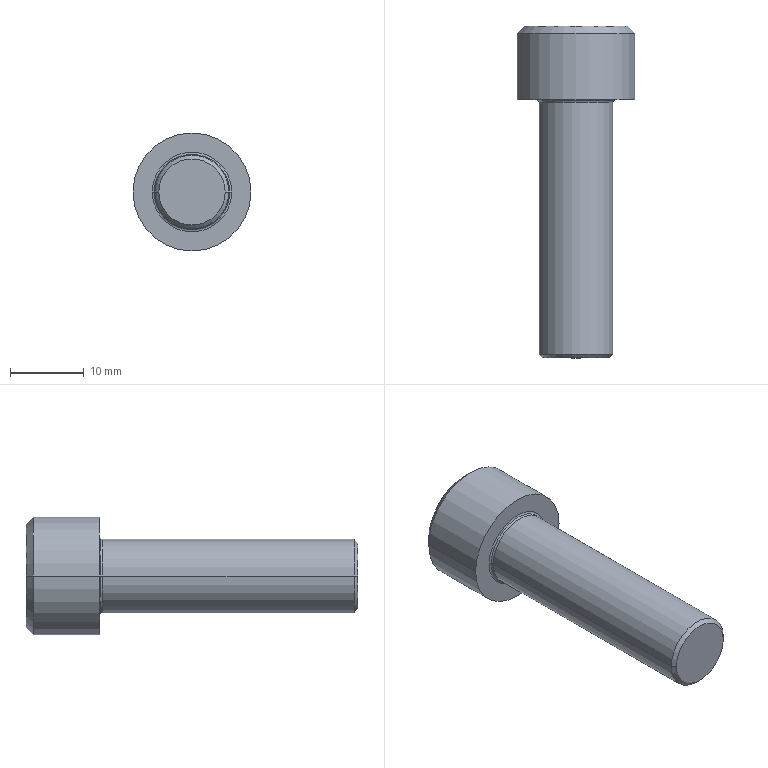Part | Creo | 1 solid | 23 faces | box 16 x 45 x 16 mm | volume 4398 mm3 | plane 9 | cone 6 | cylinder 4 | torus 4 | commonest cylinder face diameters 10 x2 16 x2
STEP:
#1=CARTESIAN_POINT('',(-187.881,357.995,-225.));
#2=VERTEX_POINT('',#1);
#3=CARTESIAN_POINT('',(-190.191,357.995,-229.));
#4=VERTEX_POINT('',#3);
#5=CARTESIAN_POINT('',(-187.881,357.995,-225.));
#6=CARTESIAN_POINT('',(-187.989,357.933,-225.187));
#7=CARTESIAN_POINT('',(-188.205,357.821,-225.561));
#8=CARTESIAN_POINT('',(-188.534,357.7,-226.131));
#9=CARTESIAN_POINT('',(-188.867,357.635,-226.708));
#10=CARTESIAN_POINT('',(-189.204,357.635,-227.29));
#11=CARTESIAN_POINT('',(-189.537,357.7,-227.868));
#12=CARTESIAN_POINT('',(-189.865,357.821,-228.437));
#13=CARTESIAN_POINT('',(-190.082,357.933,-228.813));
#14=CARTESIAN_POINT('',(-190.191,357.995,-229.));
#15=B_SPLINE_CURVE_WITH_KNOTS('',3,(#5,#6,#7,#8,#9,#10,#11,#12,#13,#14),.UNSPECIFIED.,.F.,.F.,(4,1,1,1,1,1,1,4),(0.,0.1429,0.2857,0.4286,0.5714,0.7143,0.8571,1.),.UNSPECIFIED.);
#16=EDGE_CURVE('',#2,#4,#15,.T.);
#17=ORIENTED_EDGE('',*,*,#16,.F.);
#18=CARTESIAN_POINT('',(-192.5,355.329,-225.));
#19=VERTEX_POINT('',#18);
#20=CARTESIAN_POINT('',(-192.5,355.329,-225.));
#21=DIRECTION('',(0.866,0.5,0.));
#22=VECTOR('',#21,5.333);
#23=LINE('',#20,#22);
#24=EDGE_CURVE('',#19,#2,#23,.T.);
#25=ORIENTED_EDGE('',*,*,#24,.F.);
#26=CARTESIAN_POINT('',(-197.119,357.995,-225.));
#27=VERTEX_POINT('',#26);
#28=CARTESIAN_POINT('',(-192.5,355.329,-225.));
#29=DIRECTION('',(-0.866,0.5,0.));
#30=VECTOR('',#29,5.333);
#31=LINE('',#28,#30);
#32=EDGE_CURVE('',#19,#27,#31,.T.);
#33=ORIENTED_EDGE('',*,*,#32,.T.);
#34=CARTESIAN_POINT('',(-194.809,357.995,-229.));
#35=VERTEX_POINT('',#34);
#36=CARTESIAN_POINT('',(-194.809,357.995,-229.));
#37=CARTESIAN_POINT('',(-194.917,357.933,-228.813));
#38=CARTESIAN_POINT('',(-195.133,357.821,-228.439));
#39=CARTESIAN_POINT('',(-195.462,357.7,-227.869));
#40=CARTESIAN_POINT('',(-195.795,357.635,-227.292));
#41=CARTESIAN_POINT('',(-196.132,357.635,-226.71));
#42=CARTESIAN_POINT('',(-196.465,357.7,-226.132));
#43=CARTESIAN_POINT('',(-196.794,357.821,-225.563));
#44=CARTESIAN_POINT('',(-197.011,357.933,-225.187));
#45=CARTESIAN_POINT('',(-197.119,357.995,-225.));
#46=B_SPLINE_CURVE_WITH_KNOTS('',3,(#36,#37,#38,#39,#40,#41,#42,#43,#44,#45),.UNSPECIFIED.,.F.,.F.,(4,1,1,1,1,1,1,4),(0.,0.1429,0.2857,0.4286,0.5714,0.7143,0.8571,1.),.UNSPECIFIED.);
#47=EDGE_CURVE('',#35,#27,#46,.T.);
#48=ORIENTED_EDGE('',*,*,#47,.F.);
#49=CARTESIAN_POINT('',(-190.191,357.995,-229.));
#50=CARTESIAN_POINT('',(-190.404,357.934,-229.));
#51=CARTESIAN_POINT('',(-190.835,357.822,-229.));
#52=CARTESIAN_POINT('',(-191.496,357.7,-229.));
#53=CARTESIAN_POINT('',(-192.165,357.635,-229.));
#54=CARTESIAN_POINT('',(-192.833,357.635,-229.));
#55=CARTESIAN_POINT('',(-193.5,357.699,-229.));
#56=CARTESIAN_POINT('',(-194.162,357.821,-229.));
#57=CARTESIAN_POINT('',(-194.594,357.933,-229.));
#58=CARTESIAN_POINT('',(-194.809,357.995,-229.));
#59=B_SPLINE_CURVE_WITH_KNOTS('',3,(#49,#50,#51,#52,#53,#54,#55,#56,#57,#58),.UNSPECIFIED.,.F.,.F.,(4,1,1,1,1,1,1,4),(0.,0.1429,0.2857,0.4286,0.5714,0.7143,0.8571,1.),.UNSPECIFIED.);
#60=EDGE_CURVE('',#4,#35,#59,.T.);
#61=ORIENTED_EDGE('',*,*,#60,.F.);
#62=EDGE_LOOP('',(#17,#25,#33,#48,#61));
#63=FACE_OUTER_BOUND('',#62,.F.);
#64=CARTESIAN_POINT('',(-192.5,356.689,-225.));
#65=DIRECTION('',(0.,1.,0.));
#66=DIRECTION('',(1.,0.,0.));
#67=AXIS2_PLACEMENT_3D('',#64,#65,#66);
#68=CONICAL_SURFACE('',#67,2.356,60.);
#69=ADVANCED_FACE('',(#63),#68,.F.);
#70=CARTESIAN_POINT('',(-190.191,362.995,-229.));
#71=VERTEX_POINT('',#70);
#72=CARTESIAN_POINT('',(-187.881,362.995,-225.));
#73=VERTEX_POINT('',#72);
#74=CARTESIAN_POINT('',(-190.191,362.995,-229.));
#75=DIRECTION('',(0.5,0.,0.866));
#76=VECTOR('',#75,4.619);
#77=LINE('',#74,#76);
#78=EDGE_CURVE('',#71,#73,#77,.T.);
#79=ORIENTED_EDGE('',*,*,#78,.T.);
#80=CARTESIAN_POINT('',(-187.881,362.995,-225.));
#81=DIRECTION('',(0.,-1.,0.));
#82=VECTOR('',#81,5.);
#83=LINE('',#80,#82);
#84=EDGE_CURVE('',#73,#2,#83,.T.);
#85=ORIENTED_EDGE('',*,*,#84,.T.);
#86=ORIENTED_EDGE('',*,*,#16,.T.);
#87=CARTESIAN_POINT('',(-190.191,362.995,-229.));
#88=DIRECTION('',(0.,-1.,0.));
#89=VECTOR('',#88,5.);
#90=LINE('',#87,#89);
#91=EDGE_CURVE('',#71,#4,#90,.T.);
#92=ORIENTED_EDGE('',*,*,#91,.F.);
#93=EDGE_LOOP('',(#79,#85,#86,#92));
#94=FACE_OUTER_BOUND('',#93,.F.);
#95=CARTESIAN_POINT('',(-190.191,357.995,-229.));
#96=DIRECTION('',(-0.866,0.,0.5));
#97=DIRECTION('',(0.5,0.,0.866));
#98=AXIS2_PLACEMENT_3D('',#95,#96,#97);
#99=PLANE('',#98);
#100=ADVANCED_FACE('',(#94),#99,.T.);
#101=CARTESIAN_POINT('',(-185.5,362.995,-225.));
#102=VERTEX_POINT('',#101);
#103=CARTESIAN_POINT('',(-199.5,362.995,-225.));
#104=VERTEX_POINT('',#103);
#105=CARTESIAN_POINT('',(-192.5,362.995,-225.));
#106=DIRECTION('',(0.,1.,0.));
#107=DIRECTION('',(1.,0.,0.));
#108=AXIS2_PLACEMENT_3D('',#105,#106,#107);
#109=CIRCLE('',#108,7.);
#110=EDGE_CURVE('',#102,#104,#109,.T.);
#111=ORIENTED_EDGE('',*,*,#110,.F.);
#112=CARTESIAN_POINT('',(-192.5,362.995,-225.));
#113=DIRECTION('',(0.,1.,0.));
#114=DIRECTION('',(-1.,0.,0.));
#115=AXIS2_PLACEMENT_3D('',#112,#113,#114);
#116=CIRCLE('',#115,7.);
#117=EDGE_CURVE('',#104,#102,#116,.T.);
#118=ORIENTED_EDGE('',*,*,#117,.F.);
#119=EDGE_LOOP('',(#111,#118));
#120=FACE_OUTER_BOUND('',#119,.F.);
#121=CARTESIAN_POINT('',(-190.191,362.995,-221.));
#122=VERTEX_POINT('',#121);
#123=CARTESIAN_POINT('',(-187.881,362.995,-225.));
#124=DIRECTION('',(-0.5,0.,0.866));
#125=VECTOR('',#124,4.619);
#126=LINE('',#123,#125);
#127=EDGE_CURVE('',#73,#122,#126,.T.);
#128=ORIENTED_EDGE('',*,*,#127,.F.);
#129=ORIENTED_EDGE('',*,*,#78,.F.);
#130=CARTESIAN_POINT('',(-194.809,362.995,-229.));
#131=VERTEX_POINT('',#130);
#132=CARTESIAN_POINT('',(-190.191,362.995,-229.));
#133=DIRECTION('',(-1.,0.,0.));
#134=VECTOR('',#133,4.619);
#135=LINE('',#132,#134);
#136=EDGE_CURVE('',#71,#131,#135,.T.);
#137=ORIENTED_EDGE('',*,*,#136,.T.);
#138=CARTESIAN_POINT('',(-197.119,362.995,-225.));
#139=VERTEX_POINT('',#138);
#140=CARTESIAN_POINT('',(-197.119,362.995,-225.));
#141=DIRECTION('',(0.5,0.,-0.866));
#142=VECTOR('',#141,4.619);
#143=LINE('',#140,#142);
#144=EDGE_CURVE('',#139,#131,#143,.T.);
#145=ORIENTED_EDGE('',*,*,#144,.F.);
#146=CARTESIAN_POINT('',(-194.809,362.995,-221.));
#147=VERTEX_POINT('',#146);
#148=CARTESIAN_POINT('',(-194.809,362.995,-221.));
#149=DIRECTION('',(-0.5,0.,-0.866));
#150=VECTOR('',#149,4.619);
#151=LINE('',#148,#150);
#152=EDGE_CURVE('',#147,#139,#151,.T.);
#153=ORIENTED_EDGE('',*,*,#152,.F.);
#154=CARTESIAN_POINT('',(-194.809,362.995,-221.));
#155=DIRECTION('',(1.,0.,0.));
#156=VECTOR('',#155,4.619);
#157=LINE('',#154,#156);
#158=EDGE_CURVE('',#147,#122,#157,.T.);
#159=ORIENTED_EDGE('',*,*,#158,.T.);
#160=EDGE_LOOP('',(#128,#129,#137,#145,#153,#159));
#161=FACE_BOUND('',#160,.F.);
#162=CARTESIAN_POINT('',(-192.5,362.995,-225.));
#163=DIRECTION('',(0.,1.,0.));
#164=DIRECTION('',(1.,0.,0.));
#165=AXIS2_PLACEMENT_3D('',#162,#163,#164);
#166=PLANE('',#165);
#167=ADVANCED_FACE('',(#120,#161),#166,.T.);
#168=CARTESIAN_POINT('',(-184.5,361.995,-225.));
#169=VERTEX_POINT('',#168);
#170=CARTESIAN_POINT('',(-200.5,361.995,-225.));
#171=VERTEX_POINT('',#170);
#172=CARTESIAN_POINT('',(-192.5,361.995,-225.));
#173=DIRECTION('',(0.,1.,0.));
#174=DIRECTION('',(1.,0.,0.));
#175=AXIS2_PLACEMENT_3D('',#172,#173,#174);
#176=CIRCLE('',#175,8.);
#177=EDGE_CURVE('',#169,#171,#176,.T.);
#178=ORIENTED_EDGE('',*,*,#177,.F.);
#179=CARTESIAN_POINT('',(-185.5,362.995,-225.));
#180=DIRECTION('',(0.7071,-0.7071,0.));
#181=VECTOR('',#180,1.414);
#182=LINE('',#179,#181);
#183=EDGE_CURVE('',#102,#169,#182,.T.);
#184=ORIENTED_EDGE('',*,*,#183,.F.);
#185=ORIENTED_EDGE('',*,*,#110,.T.);
#186=CARTESIAN_POINT('',(-199.5,362.995,-225.));
#187=DIRECTION('',(-0.7071,-0.7071,0.));
#188=VECTOR('',#187,1.414);
#189=LINE('',#186,#188);
#190=EDGE_CURVE('',#104,#171,#189,.T.);
#191=ORIENTED_EDGE('',*,*,#190,.T.);
#192=EDGE_LOOP('',(#178,#184,#185,#191));
#193=FACE_OUTER_BOUND('',#192,.F.);
#194=CARTESIAN_POINT('',(-192.5,362.495,-225.));
#195=DIRECTION('',(0.,-1.,0.));
#196=DIRECTION('',(-1.,0.,0.));
#197=AXIS2_PLACEMENT_3D('',#194,#195,#196);
#198=CONICAL_SURFACE('',#197,7.5,45.);
#199=ADVANCED_FACE('',(#193),#198,.T.);
#200=ORIENTED_EDGE('',*,*,#177,.T.);
#201=CARTESIAN_POINT('',(-200.5,352.995,-225.));
#202=VERTEX_POINT('',#201);
#203=CARTESIAN_POINT('',(-200.5,352.995,-225.));
#204=DIRECTION('',(0.,1.,0.));
#205=VECTOR('',#204,9.);
#206=LINE('',#203,#205);
#207=EDGE_CURVE('',#202,#171,#206,.T.);
#208=ORIENTED_EDGE('',*,*,#207,.F.);
#209=CARTESIAN_POINT('',(-184.5,352.995,-225.));
#210=VERTEX_POINT('',#209);
#211=CARTESIAN_POINT('',(-192.5,352.995,-225.));
#212=DIRECTION('',(0.,-1.,0.));
#213=DIRECTION('',(-1.,0.,0.));
#214=AXIS2_PLACEMENT_3D('',#211,#212,#213);
#215=CIRCLE('',#214,8.);
#216=EDGE_CURVE('',#202,#210,#215,.T.);
#217=ORIENTED_EDGE('',*,*,#216,.T.);
#218=CARTESIAN_POINT('',(-184.5,352.995,-225.));
#219=DIRECTION('',(0.,1.,0.));
#220=VECTOR('',#219,9.);
#221=LINE('',#218,#220);
#222=EDGE_CURVE('',#210,#169,#221,.T.);
#223=ORIENTED_EDGE('',*,*,#222,.T.);
#224=EDGE_LOOP('',(#200,#208,#217,#223));
#225=FACE_OUTER_BOUND('',#224,.F.);
#226=CARTESIAN_POINT('',(-192.5,352.995,-225.));
#227=DIRECTION('',(0.,1.,0.));
#228=DIRECTION('',(1.,0.,0.));
#229=AXIS2_PLACEMENT_3D('',#226,#227,#228);
#230=CYLINDRICAL_SURFACE('',#229,8.);
#231=ADVANCED_FACE('',(#225),#230,.T.);
#232=CARTESIAN_POINT('',(-192.5,361.995,-225.));
#233=DIRECTION('',(0.,1.,0.));
#234=DIRECTION('',(-1.,0.,0.));
#235=AXIS2_PLACEMENT_3D('',#232,#233,#234);
#236=CIRCLE('',#235,8.);
#237=EDGE_CURVE('',#171,#169,#236,.T.);
#238=ORIENTED_EDGE('',*,*,#237,.T.);
#239=ORIENTED_EDGE('',*,*,#222,.F.);
#240=CARTESIAN_POINT('',(-192.5,352.995,-225.));
#241=DIRECTION('',(0.,-1.,0.));
#242=DIRECTION('',(1.,0.,0.));
#243=AXIS2_PLACEMENT_3D('',#240,#241,#242);
#244=CIRCLE('',#243,8.);
#245=EDGE_CURVE('',#210,#202,#244,.T.);
#246=ORIENTED_EDGE('',*,*,#245,.T.);
#247=ORIENTED_EDGE('',*,*,#207,.T.);
#248=EDGE_LOOP('',(#238,#239,#246,#247));
#249=FACE_OUTER_BOUND('',#248,.F.);
#250=CARTESIAN_POINT('',(-192.5,352.995,-225.));
#251=DIRECTION('',(0.,1.,0.));
#252=DIRECTION('',(1.,0.,0.));
#253=AXIS2_PLACEMENT_3D('',#250,#251,#252);
#254=CYLINDRICAL_SURFACE('',#253,8.);
#255=ADVANCED_FACE('',(#249),#254,.T.);
#256=ORIENTED_EDGE('',*,*,#237,.F.);
#257=ORIENTED_EDGE('',*,*,#190,.F.);
#258=ORIENTED_EDGE('',*,*,#117,.T.);
#259=ORIENTED_EDGE('',*,*,#183,.T.);
#260=EDGE_LOOP('',(#256,#257,#258,#259));
#261=FACE_OUTER_BOUND('',#260,.F.);
#262=CARTESIAN_POINT('',(-192.5,362.495,-225.));
#263=DIRECTION('',(0.,-1.,0.));
#264=DIRECTION('',(-1.,0.,0.));
#265=AXIS2_PLACEMENT_3D('',#262,#263,#264);
#266=CONICAL_SURFACE('',#265,7.5,45.);
#267=ADVANCED_FACE('',(#261),#266,.T.);
#268=ORIENTED_EDGE('',*,*,#245,.F.);
#269=ORIENTED_EDGE('',*,*,#216,.F.);
#270=EDGE_LOOP('',(#268,#269));
#271=FACE_OUTER_BOUND('',#270,.F.);
#272=CARTESIAN_POINT('',(-187.1,352.995,-225.));
#273=VERTEX_POINT('',#272);
#274=CARTESIAN_POINT('',(-197.9,352.995,-225.));
#275=VERTEX_POINT('',#274);
#276=CARTESIAN_POINT('',(-192.5,352.995,-225.));
#277=DIRECTION('',(0.,1.,0.));
#278=DIRECTION('',(1.,0.,0.));
#279=AXIS2_PLACEMENT_3D('',#276,#277,#278);
#280=CIRCLE('',#279,5.4);
#281=EDGE_CURVE('',#273,#275,#280,.T.);
#282=ORIENTED_EDGE('',*,*,#281,.F.);
#283=CARTESIAN_POINT('',(-192.5,352.995,-225.));
#284=DIRECTION('',(0.,1.,0.));
#285=DIRECTION('',(-1.,0.,0.));
#286=AXIS2_PLACEMENT_3D('',#283,#284,#285);
#287=CIRCLE('',#286,5.4);
#288=EDGE_CURVE('',#275,#273,#287,.T.);
#289=ORIENTED_EDGE('',*,*,#288,.F.);
#290=EDGE_LOOP('',(#282,#289));
#291=FACE_BOUND('',#290,.F.);
#292=CARTESIAN_POINT('',(-192.5,352.995,-225.));
#293=DIRECTION('',(0.,1.,0.));
#294=DIRECTION('',(1.,0.,0.));
#295=AXIS2_PLACEMENT_3D('',#292,#293,#294);
#296=PLANE('',#295);
#297=ADVANCED_FACE('',(#271,#291),#296,.F.);
#298=ORIENTED_EDGE('',*,*,#281,.T.);
#299=CARTESIAN_POINT('',(-197.617,352.878,-225.));
#300=VERTEX_POINT('',#299);
#301=CARTESIAN_POINT('',(-197.9,352.595,-225.));
#302=DIRECTION('',(0.,0.,-1.));
#303=DIRECTION('',(0.,1.,0.));
#304=AXIS2_PLACEMENT_3D('',#301,#302,#303);
#305=CIRCLE('',#304,0.4);
#306=EDGE_CURVE('',#275,#300,#305,.T.);
#307=ORIENTED_EDGE('',*,*,#306,.T.);
#308=CARTESIAN_POINT('',(-187.383,352.878,-225.));
#309=VERTEX_POINT('',#308);
#310=CARTESIAN_POINT('',(-192.5,352.878,-225.));
#311=DIRECTION('',(0.,1.,0.));
#312=DIRECTION('',(1.,0.,0.));
#313=AXIS2_PLACEMENT_3D('',#310,#311,#312);
#314=CIRCLE('',#313,5.117);
#315=EDGE_CURVE('',#309,#300,#314,.T.);
#316=ORIENTED_EDGE('',*,*,#315,.F.);
#317=CARTESIAN_POINT('',(-187.1,352.595,-225.));
#318=DIRECTION('',(0.,0.,1.));
#319=DIRECTION('',(0.,1.,0.));
#320=AXIS2_PLACEMENT_3D('',#317,#318,#319);
#321=CIRCLE('',#320,0.4);
#322=EDGE_CURVE('',#273,#309,#321,.T.);
#323=ORIENTED_EDGE('',*,*,#322,.F.);
#324=EDGE_LOOP('',(#298,#307,#316,#323));
#325=FACE_OUTER_BOUND('',#324,.F.);
#326=CARTESIAN_POINT('',(-192.5,352.595,-225.));
#327=DIRECTION('',(0.,1.,0.));
#328=DIRECTION('',(1.,0.,0.));
#329=AXIS2_PLACEMENT_3D('',#326,#327,#328);
#330=TOROIDAL_SURFACE('',#329,5.4,0.4);
#331=ADVANCED_FACE('',(#325),#330,.F.);
#332=ORIENTED_EDGE('',*,*,#288,.T.);
#333=ORIENTED_EDGE('',*,*,#322,.T.);
#334=CARTESIAN_POINT('',(-192.5,352.878,-225.));
#335=DIRECTION('',(0.,1.,0.));
#336=DIRECTION('',(-1.,0.,0.));
#337=AXIS2_PLACEMENT_3D('',#334,#335,#336);
#338=CIRCLE('',#337,5.117);
#339=EDGE_CURVE('',#300,#309,#338,.T.);
#340=ORIENTED_EDGE('',*,*,#339,.F.);
#341=ORIENTED_EDGE('',*,*,#306,.F.);
#342=EDGE_LOOP('',(#332,#333,#340,#341));
#343=FACE_OUTER_BOUND('',#342,.F.);
#344=CARTESIAN_POINT('',(-192.5,352.595,-225.));
#345=DIRECTION('',(0.,1.,0.));
#346=DIRECTION('',(1.,0.,0.));
#347=AXIS2_PLACEMENT_3D('',#344,#345,#346);
#348=TOROIDAL_SURFACE('',#347,5.4,0.4);
#349=ADVANCED_FACE('',(#343),#348,.F.);
#350=CARTESIAN_POINT('',(-197.5,352.595,-225.));
#351=VERTEX_POINT('',#350);
#352=CARTESIAN_POINT('',(-187.5,352.595,-225.));
#353=VERTEX_POINT('',#352);
#354=CARTESIAN_POINT('',(-192.5,352.595,-225.));
#355=DIRECTION('',(0.,1.,0.));
#356=DIRECTION('',(-1.,0.,0.));
#357=AXIS2_PLACEMENT_3D('',#354,#355,#356);
#358=CIRCLE('',#357,5.);
#359=EDGE_CURVE('',#351,#353,#358,.T.);
#360=ORIENTED_EDGE('',*,*,#359,.F.);
#361=CARTESIAN_POINT('',(-197.9,352.595,-225.));
#362=DIRECTION('',(0.,0.,-1.));
#363=DIRECTION('',(0.7071,0.7071,0.));
#364=AXIS2_PLACEMENT_3D('',#361,#362,#363);
#365=CIRCLE('',#364,0.4);
#366=EDGE_CURVE('',#300,#351,#365,.T.);
#367=ORIENTED_EDGE('',*,*,#366,.F.);
#368=ORIENTED_EDGE('',*,*,#339,.T.);
#369=CARTESIAN_POINT('',(-187.1,352.595,-225.));
#370=DIRECTION('',(0.,0.,1.));
#371=DIRECTION('',(-0.7071,0.7071,0.));
#372=AXIS2_PLACEMENT_3D('',#369,#370,#371);
#373=CIRCLE('',#372,0.4);
#374=EDGE_CURVE('',#309,#353,#373,.T.);
#375=ORIENTED_EDGE('',*,*,#374,.T.);
#376=EDGE_LOOP('',(#360,#367,#368,#375));
#377=FACE_OUTER_BOUND('',#376,.F.);
#378=CARTESIAN_POINT('',(-192.5,352.595,-225.));
#379=DIRECTION('',(0.,1.,0.));
#380=DIRECTION('',(1.,0.,0.));
#381=AXIS2_PLACEMENT_3D('',#378,#379,#380);
#382=TOROIDAL_SURFACE('',#381,5.4,0.4);
#383=ADVANCED_FACE('',(#377),#382,.F.);
#384=CARTESIAN_POINT('',(-187.5,318.495,-225.));
#385=VERTEX_POINT('',#384);
#386=CARTESIAN_POINT('',(-197.5,318.495,-225.));
#387=VERTEX_POINT('',#386);
#388=CARTESIAN_POINT('',(-192.5,318.495,-225.));
#389=DIRECTION('',(0.,-1.,0.));
#390=DIRECTION('',(1.,0.,0.));
#391=AXIS2_PLACEMENT_3D('',#388,#389,#390);
#392=CIRCLE('',#391,5.);
#393=EDGE_CURVE('',#385,#387,#392,.T.);
#394=ORIENTED_EDGE('',*,*,#393,.T.);
#395=CARTESIAN_POINT('',(-197.5,318.495,-225.));
#396=DIRECTION('',(0.,1.,0.));
#397=VECTOR('',#396,34.1);
#398=LINE('',#395,#397);
#399=EDGE_CURVE('',#387,#351,#398,.T.);
#400=ORIENTED_EDGE('',*,*,#399,.T.);
#401=ORIENTED_EDGE('',*,*,#359,.T.);
#402=CARTESIAN_POINT('',(-187.5,318.495,-225.));
#403=DIRECTION('',(0.,1.,0.));
#404=VECTOR('',#403,34.1);
#405=LINE('',#402,#404);
#406=EDGE_CURVE('',#385,#353,#405,.T.);
#407=ORIENTED_EDGE('',*,*,#406,.F.);
#408=EDGE_LOOP('',(#394,#400,#401,#407));
#409=FACE_OUTER_BOUND('',#408,.F.);
#410=CARTESIAN_POINT('',(-192.5,317.995,-225.));
#411=DIRECTION('',(0.,1.,0.));
#412=DIRECTION('',(1.,0.,0.));
#413=AXIS2_PLACEMENT_3D('',#410,#411,#412);
#414=CYLINDRICAL_SURFACE('',#413,5.);
#415=ADVANCED_FACE('',(#409),#414,.T.);
#416=CARTESIAN_POINT('',(-188.,317.995,-225.));
#417=VERTEX_POINT('',#416);
#418=CARTESIAN_POINT('',(-197.,317.995,-225.));
#419=VERTEX_POINT('',#418);
#420=CARTESIAN_POINT('',(-192.5,317.995,-225.));
#421=DIRECTION('',(0.,-1.,0.));
#422=DIRECTION('',(1.,0.,0.));
#423=AXIS2_PLACEMENT_3D('',#420,#421,#422);
#424=CIRCLE('',#423,4.5);
#425=EDGE_CURVE('',#417,#419,#424,.T.);
#426=ORIENTED_EDGE('',*,*,#425,.T.);
#427=CARTESIAN_POINT('',(-197.,317.995,-225.));
#428=DIRECTION('',(-0.7071,0.7071,0.));
#429=VECTOR('',#428,0.7071);
#430=LINE('',#427,#429);
#431=EDGE_CURVE('',#419,#387,#430,.T.);
#432=ORIENTED_EDGE('',*,*,#431,.T.);
#433=ORIENTED_EDGE('',*,*,#393,.F.);
#434=CARTESIAN_POINT('',(-188.,317.995,-225.));
#435=DIRECTION('',(0.7071,0.7071,0.));
#436=VECTOR('',#435,0.7071);
#437=LINE('',#434,#436);
#438=EDGE_CURVE('',#417,#385,#437,.T.);
#439=ORIENTED_EDGE('',*,*,#438,.F.);
#440=EDGE_LOOP('',(#426,#432,#433,#439));
#441=FACE_OUTER_BOUND('',#440,.F.);
#442=CARTESIAN_POINT('',(-192.5,318.245,-225.));
#443=DIRECTION('',(0.,1.,0.));
#444=DIRECTION('',(1.,0.,0.));
#445=AXIS2_PLACEMENT_3D('',#442,#443,#444);
#446=CONICAL_SURFACE('',#445,4.75,45.);
#447=ADVANCED_FACE('',(#441),#446,.T.);
#448=ORIENTED_EDGE('',*,*,#425,.F.);
#449=CARTESIAN_POINT('',(-192.5,317.995,-225.));
#450=DIRECTION('',(0.,-1.,0.));
#451=DIRECTION('',(-1.,0.,0.));
#452=AXIS2_PLACEMENT_3D('',#449,#450,#451);
#453=CIRCLE('',#452,4.5);
#454=EDGE_CURVE('',#419,#417,#453,.T.);
#455=ORIENTED_EDGE('',*,*,#454,.F.);
#456=EDGE_LOOP('',(#448,#455));
#457=FACE_OUTER_BOUND('',#456,.F.);
#458=CARTESIAN_POINT('',(-192.5,317.995,-225.));
#459=DIRECTION('',(0.,1.,0.));
#460=DIRECTION('',(1.,0.,0.));
#461=AXIS2_PLACEMENT_3D('',#458,#459,#460);
#462=PLANE('',#461);
#463=ADVANCED_FACE('',(#457),#462,.F.);
#464=ORIENTED_EDGE('',*,*,#454,.T.);
#465=ORIENTED_EDGE('',*,*,#438,.T.);
#466=CARTESIAN_POINT('',(-192.5,318.495,-225.));
#467=DIRECTION('',(0.,-1.,0.));
#468=DIRECTION('',(-1.,0.,0.));
#469=AXIS2_PLACEMENT_3D('',#466,#467,#468);
#470=CIRCLE('',#469,5.);
#471=EDGE_CURVE('',#387,#385,#470,.T.);
#472=ORIENTED_EDGE('',*,*,#471,.F.);
#473=ORIENTED_EDGE('',*,*,#431,.F.);
#474=EDGE_LOOP('',(#464,#465,#472,#473));
#475=FACE_OUTER_BOUND('',#474,.F.);
#476=CARTESIAN_POINT('',(-192.5,318.245,-225.));
#477=DIRECTION('',(0.,1.,0.));
#478=DIRECTION('',(1.,0.,0.));
#479=AXIS2_PLACEMENT_3D('',#476,#477,#478);
#480=CONICAL_SURFACE('',#479,4.75,45.);
#481=ADVANCED_FACE('',(#475),#480,.T.);
#482=ORIENTED_EDGE('',*,*,#471,.T.);
#483=ORIENTED_EDGE('',*,*,#406,.T.);
#484=CARTESIAN_POINT('',(-192.5,352.595,-225.));
#485=DIRECTION('',(0.,1.,0.));
#486=DIRECTION('',(1.,0.,0.));
#487=AXIS2_PLACEMENT_3D('',#484,#485,#486);
#488=CIRCLE('',#487,5.);
#489=EDGE_CURVE('',#353,#351,#488,.T.);
#490=ORIENTED_EDGE('',*,*,#489,.T.);
#491=ORIENTED_EDGE('',*,*,#399,.F.);
#492=EDGE_LOOP('',(#482,#483,#490,#491));
#493=FACE_OUTER_BOUND('',#492,.F.);
#494=CARTESIAN_POINT('',(-192.5,317.995,-225.));
#495=DIRECTION('',(0.,1.,0.));
#496=DIRECTION('',(1.,0.,0.));
#497=AXIS2_PLACEMENT_3D('',#494,#495,#496);
#498=CYLINDRICAL_SURFACE('',#497,5.);
#499=ADVANCED_FACE('',(#493),#498,.T.);
#500=ORIENTED_EDGE('',*,*,#489,.F.);
#501=ORIENTED_EDGE('',*,*,#374,.F.);
#502=ORIENTED_EDGE('',*,*,#315,.T.);
#503=ORIENTED_EDGE('',*,*,#366,.T.);
#504=EDGE_LOOP('',(#500,#501,#502,#503));
#505=FACE_OUTER_BOUND('',#504,.F.);
#506=CARTESIAN_POINT('',(-192.5,352.595,-225.));
#507=DIRECTION('',(0.,1.,0.));
#508=DIRECTION('',(1.,0.,0.));
#509=AXIS2_PLACEMENT_3D('',#506,#507,#508);
#510=TOROIDAL_SURFACE('',#509,5.4,0.4);
#511=ADVANCED_FACE('',(#505),#510,.F.);
#512=ORIENTED_EDGE('',*,*,#127,.T.);
#513=CARTESIAN_POINT('',(-190.191,357.995,-221.));
#514=VERTEX_POINT('',#513);
#515=CARTESIAN_POINT('',(-190.191,362.995,-221.));
#516=DIRECTION('',(0.,-1.,0.));
#517=VECTOR('',#516,5.);
#518=LINE('',#515,#517);
#519=EDGE_CURVE('',#122,#514,#518,.T.);
#520=ORIENTED_EDGE('',*,*,#519,.T.);
#521=CARTESIAN_POINT('',(-190.191,357.995,-221.));
#522=CARTESIAN_POINT('',(-190.083,357.933,-221.187));
#523=CARTESIAN_POINT('',(-189.867,357.821,-221.561));
#524=CARTESIAN_POINT('',(-189.538,357.7,-222.131));
#525=CARTESIAN_POINT('',(-189.205,357.635,-222.708));
#526=CARTESIAN_POINT('',(-188.868,357.635,-223.29));
#527=CARTESIAN_POINT('',(-188.535,357.7,-223.868));
#528=CARTESIAN_POINT('',(-188.206,357.821,-224.437));
#529=CARTESIAN_POINT('',(-187.989,357.933,-224.813));
#530=CARTESIAN_POINT('',(-187.881,357.995,-225.));
#531=B_SPLINE_CURVE_WITH_KNOTS('',3,(#521,#522,#523,#524,#525,#526,#527,#528,#529,#530),.UNSPECIFIED.,.F.,.F.,(4,1,1,1,1,1,1,4),(0.,0.1429,0.2857,0.4286,0.5714,0.7143,0.8571,1.),.UNSPECIFIED.);
#532=EDGE_CURVE('',#514,#2,#531,.T.);
#533=ORIENTED_EDGE('',*,*,#532,.T.);
#534=ORIENTED_EDGE('',*,*,#84,.F.);
#535=EDGE_LOOP('',(#512,#520,#533,#534));
#536=FACE_OUTER_BOUND('',#535,.F.);
#537=CARTESIAN_POINT('',(-187.881,357.995,-225.));
#538=DIRECTION('',(-0.866,0.,-0.5));
#539=DIRECTION('',(-0.5,0.,0.866));
#540=AXIS2_PLACEMENT_3D('',#537,#538,#539);
#541=PLANE('',#540);
#542=ADVANCED_FACE('',(#536),#541,.T.);
#543=ORIENTED_EDGE('',*,*,#158,.F.);
#544=CARTESIAN_POINT('',(-194.809,357.995,-221.));
#545=VERTEX_POINT('',#544);
#546=CARTESIAN_POINT('',(-194.809,362.995,-221.));
#547=DIRECTION('',(0.,-1.,0.));
#548=VECTOR('',#547,5.);
#549=LINE('',#546,#548);
#550=EDGE_CURVE('',#147,#545,#549,.T.);
#551=ORIENTED_EDGE('',*,*,#550,.T.);
#552=CARTESIAN_POINT('',(-194.809,357.995,-221.));
#553=CARTESIAN_POINT('',(-194.594,357.933,-221.));
#554=CARTESIAN_POINT('',(-194.162,357.821,-221.));
#555=CARTESIAN_POINT('',(-193.5,357.699,-221.));
#556=CARTESIAN_POINT('',(-192.833,357.635,-221.));
#557=CARTESIAN_POINT('',(-192.165,357.635,-221.));
#558=CARTESIAN_POINT('',(-191.496,357.7,-221.));
#559=CARTESIAN_POINT('',(-190.835,357.822,-221.));
#560=CARTESIAN_POINT('',(-190.404,357.934,-221.));
#561=CARTESIAN_POINT('',(-190.191,357.995,-221.));
#562=B_SPLINE_CURVE_WITH_KNOTS('',3,(#552,#553,#554,#555,#556,#557,#558,#559,#560,#561),.UNSPECIFIED.,.F.,.F.,(4,1,1,1,1,1,1,4),(0.,0.1429,0.2857,0.4286,0.5714,0.7143,0.8571,1.),.UNSPECIFIED.);
#563=EDGE_CURVE('',#545,#514,#562,.T.);
#564=ORIENTED_EDGE('',*,*,#563,.T.);
#565=ORIENTED_EDGE('',*,*,#519,.F.);
#566=EDGE_LOOP('',(#543,#551,#564,#565));
#567=FACE_OUTER_BOUND('',#566,.F.);
#568=CARTESIAN_POINT('',(-190.191,357.995,-221.));
#569=DIRECTION('',(0.,0.,-1.));
#570=DIRECTION('',(0.,1.,0.));
#571=AXIS2_PLACEMENT_3D('',#568,#569,#570);
#572=PLANE('',#571);
#573=ADVANCED_FACE('',(#567),#572,.T.);
#574=ORIENTED_EDGE('',*,*,#152,.T.);
#575=CARTESIAN_POINT('',(-197.119,362.995,-225.));
#576=DIRECTION('',(0.,-1.,0.));
#577=VECTOR('',#576,5.);
#578=LINE('',#575,#577);
#579=EDGE_CURVE('',#139,#27,#578,.T.);
#580=ORIENTED_EDGE('',*,*,#579,.T.);
#581=CARTESIAN_POINT('',(-197.119,357.995,-225.));
#582=CARTESIAN_POINT('',(-197.011,357.933,-224.813));
#583=CARTESIAN_POINT('',(-196.794,357.821,-224.437));
#584=CARTESIAN_POINT('',(-196.465,357.7,-223.868));
#585=CARTESIAN_POINT('',(-196.132,357.635,-223.29));
#586=CARTESIAN_POINT('',(-195.795,357.635,-222.708));
#587=CARTESIAN_POINT('',(-195.462,357.7,-222.131));
#588=CARTESIAN_POINT('',(-195.133,357.821,-221.561));
#589=CARTESIAN_POINT('',(-194.917,357.933,-221.187));
#590=CARTESIAN_POINT('',(-194.809,357.995,-221.));
#591=B_SPLINE_CURVE_WITH_KNOTS('',3,(#581,#582,#583,#584,#585,#586,#587,#588,#589,#590),.UNSPECIFIED.,.F.,.F.,(4,1,1,1,1,1,1,4),(0.,0.1429,0.2857,0.4286,0.5714,0.7143,0.8571,1.),.UNSPECIFIED.);
#592=EDGE_CURVE('',#27,#545,#591,.T.);
#593=ORIENTED_EDGE('',*,*,#592,.T.);
#594=ORIENTED_EDGE('',*,*,#550,.F.);
#595=EDGE_LOOP('',(#574,#580,#593,#594));
#596=FACE_OUTER_BOUND('',#595,.F.);
#597=CARTESIAN_POINT('',(-194.809,357.995,-221.));
#598=DIRECTION('',(0.866,0.,-0.5));
#599=DIRECTION('',(-0.5,0.,-0.866));
#600=AXIS2_PLACEMENT_3D('',#597,#598,#599);
#601=PLANE('',#600);
#602=ADVANCED_FACE('',(#596),#601,.T.);
#603=ORIENTED_EDGE('',*,*,#144,.T.);
#604=CARTESIAN_POINT('',(-194.809,362.995,-229.));
#605=DIRECTION('',(0.,-1.,0.));
#606=VECTOR('',#605,5.);
#607=LINE('',#604,#606);
#608=EDGE_CURVE('',#131,#35,#607,.T.);
#609=ORIENTED_EDGE('',*,*,#608,.T.);
#610=ORIENTED_EDGE('',*,*,#47,.T.);
#611=ORIENTED_EDGE('',*,*,#579,.F.);
#612=EDGE_LOOP('',(#603,#609,#610,#611));
#613=FACE_OUTER_BOUND('',#612,.F.);
#614=CARTESIAN_POINT('',(-197.119,357.995,-225.));
#615=DIRECTION('',(0.866,0.,0.5));
#616=DIRECTION('',(0.5,0.,-0.866));
#617=AXIS2_PLACEMENT_3D('',#614,#615,#616);
#618=PLANE('',#617);
#619=ADVANCED_FACE('',(#613),#618,.T.);
#620=ORIENTED_EDGE('',*,*,#136,.F.);
#621=ORIENTED_EDGE('',*,*,#91,.T.);
#622=ORIENTED_EDGE('',*,*,#60,.T.);
#623=ORIENTED_EDGE('',*,*,#608,.F.);
#624=EDGE_LOOP('',(#620,#621,#622,#623));
#625=FACE_OUTER_BOUND('',#624,.F.);
#626=CARTESIAN_POINT('',(-194.809,357.995,-229.));
#627=DIRECTION('',(0.,0.,1.));
#628=DIRECTION('',(0.,-1.,0.));
#629=AXIS2_PLACEMENT_3D('',#626,#627,#628);
#630=PLANE('',#629);
#631=ADVANCED_FACE('',(#625),#630,.T.);
#632=ORIENTED_EDGE('',*,*,#592,.F.);
#633=ORIENTED_EDGE('',*,*,#32,.F.);
#634=ORIENTED_EDGE('',*,*,#24,.T.);
#635=ORIENTED_EDGE('',*,*,#532,.F.);
#636=ORIENTED_EDGE('',*,*,#563,.F.);
#637=EDGE_LOOP('',(#632,#633,#634,#635,#636));
#638=FACE_OUTER_BOUND('',#637,.F.);
#639=CARTESIAN_POINT('',(-192.5,356.689,-225.));
#640=DIRECTION('',(0.,1.,0.));
#641=DIRECTION('',(1.,0.,0.));
#642=AXIS2_PLACEMENT_3D('',#639,#640,#641);
#643=CONICAL_SURFACE('',#642,2.356,60.);
#644=ADVANCED_FACE('',(#638),#643,.F.);
#645=CLOSED_SHELL('',(#69,#100,#167,#199,#231,#255,#267,#297,#331,#349,#383,#415,#447,#463,#481,#499,#511,#542,#573,#602,#619,#631,#644));
#646=MANIFOLD_SOLID_BREP('',#645);
#647=(LENGTH_UNIT()NAMED_UNIT(*)SI_UNIT(.MILLI.,.METRE.));
#648=UNCERTAINTY_MEASURE_WITH_UNIT(LENGTH_MEASURE(0.005037),#647,'','');
#649=(NAMED_UNIT(*)PLANE_ANGLE_UNIT()SI_UNIT($,.RADIAN.));
#650=PLANE_ANGLE_MEASURE_WITH_UNIT(PLANE_ANGLE_MEASURE(0.01745),#649);
#651=(CONVERSION_BASED_UNIT('DEGREE',#650)NAMED_UNIT(*)PLANE_ANGLE_UNIT());
#652=(NAMED_UNIT(*)SI_UNIT($,.STERADIAN.)SOLID_ANGLE_UNIT());
#653=(GEOMETRIC_REPRESENTATION_CONTEXT(3)GLOBAL_UNCERTAINTY_ASSIGNED_CONTEXT((#648))GLOBAL_UNIT_ASSIGNED_CONTEXT((#647,#651,#652))REPRESENTATION_CONTEXT('',''));
#654=ADVANCED_BREP_SHAPE_REPRESENTATION('',(#646),#653);